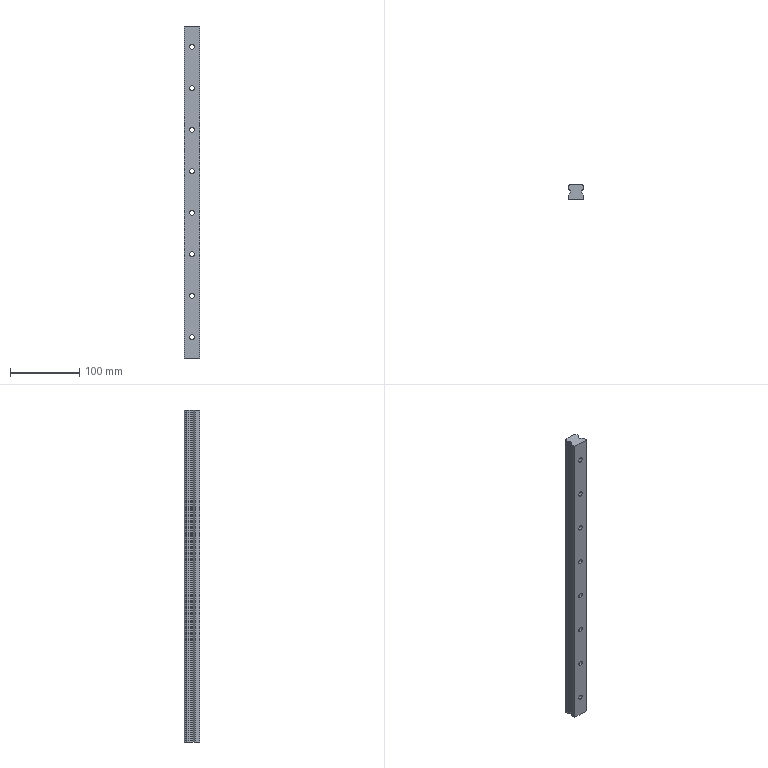Part | STEP file | 1 solid | 66 faces | box 23 x 22 x 480 mm | volume 205813 mm3 | cylinder 38 | plane 28 | commonest cylinder face diameters 7 x16 11 x16 2.258 x6